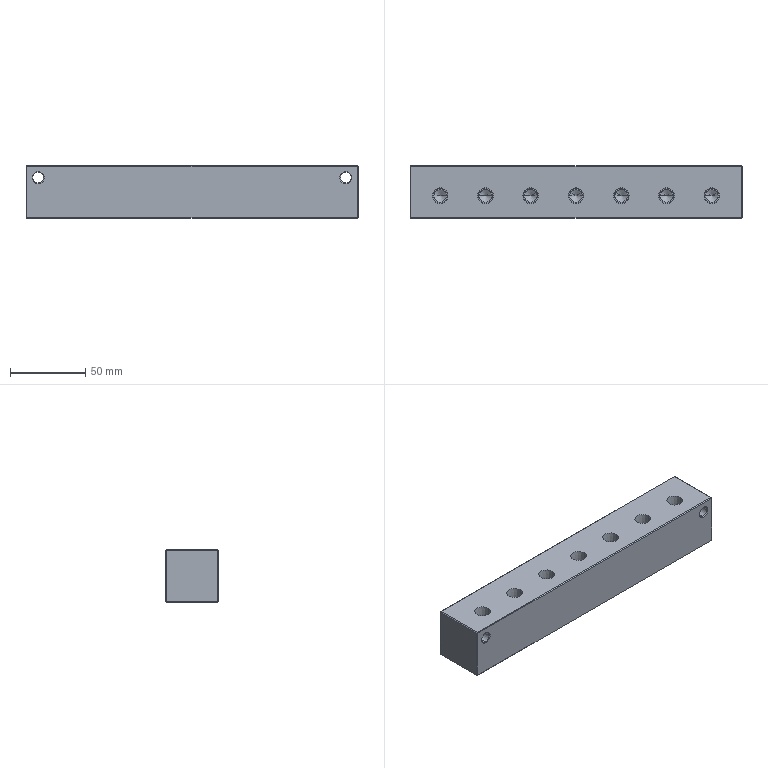Part | STEP file | OP10-010_junction block (A) | 1 solid | 135 faces | box 220 x 35 x 35 mm | volume 246704 mm3 | cone 50 | cylinder 43 | plane 42 | commonest cylinder face diameters 8.433 x35 7 x4 11 x4